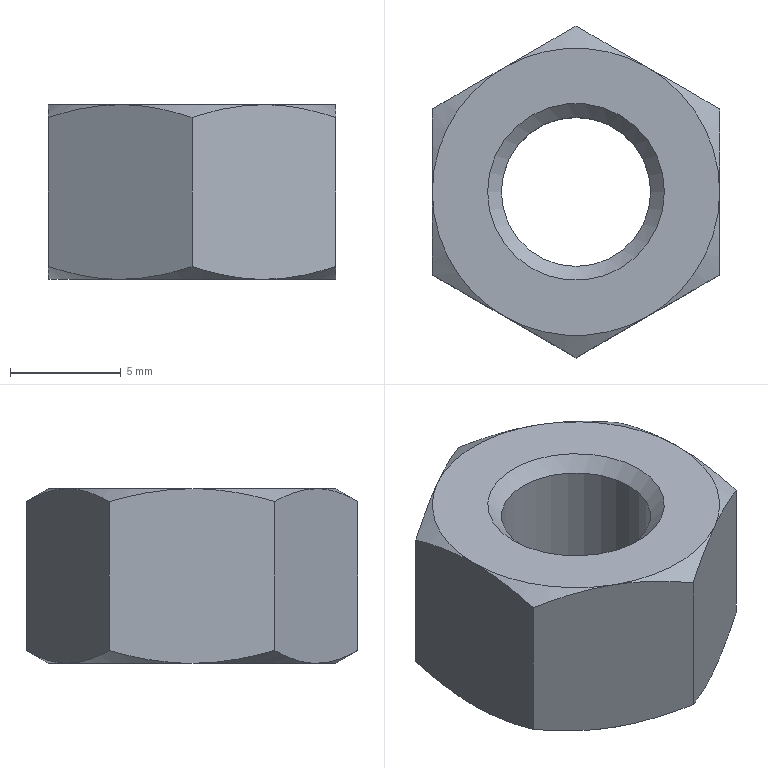Part | NX | features BREP 1, DATUM_CSYS 1 | 1 solid | 23 faces | box 13 x 15.011 x 7.9 mm | volume 859.913 mm3 | cone 14 | plane 8 | cylinder 1 | commonest cylinder face diameters 6.75 x1
STEP:
#1=CARTESIAN_POINT('',(-3.25,5.629,0.));
#2=VERTEX_POINT('',#1);
#3=CARTESIAN_POINT('',(-6.5,0.,0.));
#4=VERTEX_POINT('',#3);
#5=CARTESIAN_POINT('',(0.,0.,0.));
#6=DIRECTION('',(0.,0.,1.));
#7=DIRECTION('',(-0.5,0.866,0.));
#8=AXIS2_PLACEMENT_3D('',#5,#6,#7);
#9=CIRCLE('',#8,6.5);
#10=EDGE_CURVE('',#2,#4,#9,.T.);
#11=ORIENTED_EDGE('',*,*,#10,.F.);
#12=CARTESIAN_POINT('',(3.25,5.629,0.));
#13=VERTEX_POINT('',#12);
#14=CARTESIAN_POINT('',(0.,0.,0.));
#15=DIRECTION('',(0.,0.,1.));
#16=DIRECTION('',(0.5,0.866,0.));
#17=AXIS2_PLACEMENT_3D('',#14,#15,#16);
#18=CIRCLE('',#17,6.5);
#19=EDGE_CURVE('',#13,#2,#18,.T.);
#20=ORIENTED_EDGE('',*,*,#19,.F.);
#21=CARTESIAN_POINT('',(6.5,0.000000015,0.));
#22=VERTEX_POINT('',#21);
#23=CARTESIAN_POINT('',(0.,0.,0.));
#24=DIRECTION('',(0.,0.,1.));
#25=DIRECTION('',(1.,0.,0.));
#26=AXIS2_PLACEMENT_3D('',#23,#24,#25);
#27=CIRCLE('',#26,6.5);
#28=EDGE_CURVE('',#22,#13,#27,.T.);
#29=ORIENTED_EDGE('',*,*,#28,.F.);
#30=CARTESIAN_POINT('',(3.25,-5.629,0.));
#31=VERTEX_POINT('',#30);
#32=CARTESIAN_POINT('',(0.,0.,0.));
#33=DIRECTION('',(0.,0.,1.));
#34=DIRECTION('',(0.5,-0.866,0.));
#35=AXIS2_PLACEMENT_3D('',#32,#33,#34);
#36=CIRCLE('',#35,6.5);
#37=EDGE_CURVE('',#31,#22,#36,.T.);
#38=ORIENTED_EDGE('',*,*,#37,.F.);
#39=CARTESIAN_POINT('',(-3.25,-5.629,0.));
#40=VERTEX_POINT('',#39);
#41=CARTESIAN_POINT('',(0.,0.,0.));
#42=DIRECTION('',(0.,0.,1.));
#43=DIRECTION('',(-0.5,-0.866,0.));
#44=AXIS2_PLACEMENT_3D('',#41,#42,#43);
#45=CIRCLE('',#44,6.5);
#46=EDGE_CURVE('',#40,#31,#45,.T.);
#47=ORIENTED_EDGE('',*,*,#46,.F.);
#48=CARTESIAN_POINT('',(0.,0.,0.));
#49=DIRECTION('',(0.,0.,1.));
#50=DIRECTION('',(-1.,0.,0.));
#51=AXIS2_PLACEMENT_3D('',#48,#49,#50);
#52=CIRCLE('',#51,6.5);
#53=EDGE_CURVE('',#4,#40,#52,.T.);
#54=ORIENTED_EDGE('',*,*,#53,.F.);
#55=EDGE_LOOP('',(#11,#20,#29,#38,#47,#54));
#56=FACE_BOUND('',#55,.T.);
#57=CARTESIAN_POINT('',(4.,0.,0.));
#58=VERTEX_POINT('',#57);
#59=CARTESIAN_POINT('',(0.,0.,0.));
#60=DIRECTION('',(0.,0.,1.));
#61=DIRECTION('',(1.,0.,0.));
#62=AXIS2_PLACEMENT_3D('',#59,#60,#61);
#63=CIRCLE('',#62,4.);
#64=EDGE_CURVE('',#58,#58,#63,.T.);
#65=ORIENTED_EDGE('',*,*,#64,.T.);
#66=EDGE_LOOP('',(#65));
#67=FACE_BOUND('',#66,.T.);
#68=CARTESIAN_POINT('',(1.006,0.,0.));
#69=DIRECTION('',(0.,0.,1.));
#70=DIRECTION('',(-1.,0.,0.));
#71=AXIS2_PLACEMENT_3D('',#68,#69,#70);
#72=PLANE('',#71);
#73=ADVANCED_FACE('',(#56,#67),#72,.F.);
#74=CARTESIAN_POINT('',(6.5,0.,7.9));
#75=VERTEX_POINT('',#74);
#76=CARTESIAN_POINT('',(3.25,-5.629,7.9));
#77=VERTEX_POINT('',#76);
#78=CARTESIAN_POINT('',(0.,0.,7.9));
#79=DIRECTION('',(0.,0.,-1.));
#80=DIRECTION('',(1.,0.,0.));
#81=AXIS2_PLACEMENT_3D('',#78,#79,#80);
#82=CIRCLE('',#81,6.5);
#83=EDGE_CURVE('',#75,#77,#82,.T.);
#84=ORIENTED_EDGE('',*,*,#83,.F.);
#85=CARTESIAN_POINT('',(3.25,5.629,7.9));
#86=VERTEX_POINT('',#85);
#87=CARTESIAN_POINT('',(0.,0.,7.9));
#88=DIRECTION('',(0.,0.,-1.));
#89=DIRECTION('',(0.5,0.866,0.));
#90=AXIS2_PLACEMENT_3D('',#87,#88,#89);
#91=CIRCLE('',#90,6.5);
#92=EDGE_CURVE('',#86,#75,#91,.T.);
#93=ORIENTED_EDGE('',*,*,#92,.F.);
#94=CARTESIAN_POINT('',(-3.25,5.629,7.9));
#95=VERTEX_POINT('',#94);
#96=CARTESIAN_POINT('',(0.,0.,7.9));
#97=DIRECTION('',(0.,0.,-1.));
#98=DIRECTION('',(-0.5,0.866,0.));
#99=AXIS2_PLACEMENT_3D('',#96,#97,#98);
#100=CIRCLE('',#99,6.5);
#101=EDGE_CURVE('',#95,#86,#100,.T.);
#102=ORIENTED_EDGE('',*,*,#101,.F.);
#103=CARTESIAN_POINT('',(-6.5,0.000000016,7.9));
#104=VERTEX_POINT('',#103);
#105=CARTESIAN_POINT('',(0.,0.,7.9));
#106=DIRECTION('',(0.,0.,-1.));
#107=DIRECTION('',(-1.,0.,0.));
#108=AXIS2_PLACEMENT_3D('',#105,#106,#107);
#109=CIRCLE('',#108,6.5);
#110=EDGE_CURVE('',#104,#95,#109,.T.);
#111=ORIENTED_EDGE('',*,*,#110,.F.);
#112=CARTESIAN_POINT('',(-3.25,-5.629,7.9));
#113=VERTEX_POINT('',#112);
#114=CARTESIAN_POINT('',(0.,0.,7.9));
#115=DIRECTION('',(0.,0.,-1.));
#116=DIRECTION('',(-0.5,-0.866,0.));
#117=AXIS2_PLACEMENT_3D('',#114,#115,#116);
#118=CIRCLE('',#117,6.5);
#119=EDGE_CURVE('',#113,#104,#118,.T.);
#120=ORIENTED_EDGE('',*,*,#119,.F.);
#121=CARTESIAN_POINT('',(0.,0.,7.9));
#122=DIRECTION('',(0.,0.,-1.));
#123=DIRECTION('',(0.5,-0.866,0.));
#124=AXIS2_PLACEMENT_3D('',#121,#122,#123);
#125=CIRCLE('',#124,6.5);
#126=EDGE_CURVE('',#77,#113,#125,.T.);
#127=ORIENTED_EDGE('',*,*,#126,.F.);
#128=EDGE_LOOP('',(#84,#93,#102,#111,#120,#127));
#129=FACE_BOUND('',#128,.T.);
#130=CARTESIAN_POINT('',(4.,0.,7.9));
#131=VERTEX_POINT('',#130);
#132=CARTESIAN_POINT('',(0.,0.,7.9));
#133=DIRECTION('',(0.,0.,1.));
#134=DIRECTION('',(1.,0.,0.));
#135=AXIS2_PLACEMENT_3D('',#132,#133,#134);
#136=CIRCLE('',#135,4.);
#137=EDGE_CURVE('',#131,#131,#136,.T.);
#138=ORIENTED_EDGE('',*,*,#137,.F.);
#139=EDGE_LOOP('',(#138));
#140=FACE_BOUND('',#139,.T.);
#141=CARTESIAN_POINT('',(1.006,0.,7.9));
#142=DIRECTION('',(0.,0.,1.));
#143=DIRECTION('',(-1.,0.,0.));
#144=AXIS2_PLACEMENT_3D('',#141,#142,#143);
#145=PLANE('',#144);
#146=ADVANCED_FACE('',(#129,#140),#145,.T.);
#147=CARTESIAN_POINT('',(0.,7.506,7.319));
#148=VERTEX_POINT('',#147);
#149=CARTESIAN_POINT('',(3.25,5.629,7.9));
#150=CARTESIAN_POINT('',(2.141,6.27,7.9));
#151=CARTESIAN_POINT('',(1.062,6.892,7.673));
#152=CARTESIAN_POINT('',(0.,7.506,7.319));
#153=B_SPLINE_CURVE_WITH_KNOTS('',3,(#149,#150,#151,#152),.UNSPECIFIED.,.F.,.F.,(4,4),(0.,0.003797),.UNSPECIFIED.);
#154=EDGE_CURVE('',#86,#148,#153,.T.);
#155=ORIENTED_EDGE('',*,*,#154,.F.);
#156=CARTESIAN_POINT('',(6.5,3.753,7.319));
#157=VERTEX_POINT('',#156);
#158=CARTESIAN_POINT('',(6.5,3.753,7.319));
#159=CARTESIAN_POINT('',(5.438,4.366,7.673));
#160=CARTESIAN_POINT('',(4.359,4.989,7.9));
#161=CARTESIAN_POINT('',(3.25,5.629,7.9));
#162=B_SPLINE_CURVE_WITH_KNOTS('',3,(#158,#159,#160,#161),.UNSPECIFIED.,.F.,.F.,(4,4),(0.,0.003797),.UNSPECIFIED.);
#163=EDGE_CURVE('',#157,#86,#162,.T.);
#164=ORIENTED_EDGE('',*,*,#163,.F.);
#165=CARTESIAN_POINT('',(6.5,3.753,0.5806));
#166=VERTEX_POINT('',#165);
#167=CARTESIAN_POINT('',(6.5,3.753,0.5806));
#168=DIRECTION('',(0.,0.,1.));
#169=VECTOR('',#168,1000.);
#170=LINE('',#167,#169);
#171=EDGE_CURVE('',#166,#157,#170,.T.);
#172=ORIENTED_EDGE('',*,*,#171,.F.);
#173=CARTESIAN_POINT('',(3.25,5.629,0.));
#174=CARTESIAN_POINT('',(4.359,4.989,0.));
#175=CARTESIAN_POINT('',(5.438,4.366,0.2266));
#176=CARTESIAN_POINT('',(6.5,3.753,0.5806));
#177=B_SPLINE_CURVE_WITH_KNOTS('',3,(#173,#174,#175,#176),.UNSPECIFIED.,.F.,.F.,(4,4),(0.,0.003797),.UNSPECIFIED.);
#178=EDGE_CURVE('',#13,#166,#177,.T.);
#179=ORIENTED_EDGE('',*,*,#178,.F.);
#180=CARTESIAN_POINT('',(0.,7.506,0.5806));
#181=VERTEX_POINT('',#180);
#182=CARTESIAN_POINT('',(0.,7.506,0.5806));
#183=CARTESIAN_POINT('',(1.062,6.892,0.2266));
#184=CARTESIAN_POINT('',(2.141,6.27,0.));
#185=CARTESIAN_POINT('',(3.25,5.629,0.));
#186=B_SPLINE_CURVE_WITH_KNOTS('',3,(#182,#183,#184,#185),.UNSPECIFIED.,.F.,.F.,(4,4),(0.,0.003797),.UNSPECIFIED.);
#187=EDGE_CURVE('',#181,#13,#186,.T.);
#188=ORIENTED_EDGE('',*,*,#187,.F.);
#189=CARTESIAN_POINT('',(0.,7.506,0.5806));
#190=DIRECTION('',(0.,0.,1.));
#191=VECTOR('',#190,1000.);
#192=LINE('',#189,#191);
#193=EDGE_CURVE('',#181,#148,#192,.T.);
#194=ORIENTED_EDGE('',*,*,#193,.T.);
#195=EDGE_LOOP('',(#155,#164,#172,#179,#188,#194));
#196=FACE_BOUND('',#195,.T.);
#197=CARTESIAN_POINT('',(3.25,5.629,3.95));
#198=DIRECTION('',(0.5,0.866,0.));
#199=DIRECTION('',(0.866,-0.5,0.));
#200=AXIS2_PLACEMENT_3D('',#197,#198,#199);
#201=PLANE('',#200);
#202=ADVANCED_FACE('',(#196),#201,.T.);
#203=CARTESIAN_POINT('',(-6.5,3.753,7.319));
#204=VERTEX_POINT('',#203);
#205=CARTESIAN_POINT('',(-3.25,5.629,7.9));
#206=CARTESIAN_POINT('',(-4.359,4.989,7.9));
#207=CARTESIAN_POINT('',(-5.438,4.366,7.673));
#208=CARTESIAN_POINT('',(-6.5,3.753,7.319));
#209=B_SPLINE_CURVE_WITH_KNOTS('',3,(#205,#206,#207,#208),.UNSPECIFIED.,.F.,.F.,(4,4),(0.,0.003797),.UNSPECIFIED.);
#210=EDGE_CURVE('',#95,#204,#209,.T.);
#211=ORIENTED_EDGE('',*,*,#210,.F.);
#212=CARTESIAN_POINT('',(0.,7.506,7.319));
#213=CARTESIAN_POINT('',(-1.062,6.892,7.673));
#214=CARTESIAN_POINT('',(-2.141,6.27,7.9));
#215=CARTESIAN_POINT('',(-3.25,5.629,7.9));
#216=B_SPLINE_CURVE_WITH_KNOTS('',3,(#212,#213,#214,#215),.UNSPECIFIED.,.F.,.F.,(4,4),(0.,0.003797),.UNSPECIFIED.);
#217=EDGE_CURVE('',#148,#95,#216,.T.);
#218=ORIENTED_EDGE('',*,*,#217,.F.);
#219=ORIENTED_EDGE('',*,*,#193,.F.);
#220=CARTESIAN_POINT('',(-3.25,5.629,0.));
#221=CARTESIAN_POINT('',(-2.141,6.27,-0.000000003));
#222=CARTESIAN_POINT('',(-1.062,6.892,0.2266));
#223=CARTESIAN_POINT('',(0.,7.506,0.5806));
#224=B_SPLINE_CURVE_WITH_KNOTS('',3,(#220,#221,#222,#223),.UNSPECIFIED.,.F.,.F.,(4,4),(0.,0.003797),.UNSPECIFIED.);
#225=EDGE_CURVE('',#2,#181,#224,.T.);
#226=ORIENTED_EDGE('',*,*,#225,.F.);
#227=CARTESIAN_POINT('',(-6.5,3.753,0.5806));
#228=VERTEX_POINT('',#227);
#229=CARTESIAN_POINT('',(-6.5,3.753,0.5806));
#230=CARTESIAN_POINT('',(-5.438,4.366,0.2266));
#231=CARTESIAN_POINT('',(-4.359,4.989,0.000000003));
#232=CARTESIAN_POINT('',(-3.25,5.629,0.));
#233=B_SPLINE_CURVE_WITH_KNOTS('',3,(#229,#230,#231,#232),.UNSPECIFIED.,.F.,.F.,(4,4),(0.,0.003797),.UNSPECIFIED.);
#234=EDGE_CURVE('',#228,#2,#233,.T.);
#235=ORIENTED_EDGE('',*,*,#234,.F.);
#236=CARTESIAN_POINT('',(-6.5,3.753,0.5806));
#237=DIRECTION('',(0.,0.,1.));
#238=VECTOR('',#237,1000.);
#239=LINE('',#236,#238);
#240=EDGE_CURVE('',#228,#204,#239,.T.);
#241=ORIENTED_EDGE('',*,*,#240,.T.);
#242=EDGE_LOOP('',(#211,#218,#219,#226,#235,#241));
#243=FACE_BOUND('',#242,.T.);
#244=CARTESIAN_POINT('',(-3.25,5.629,3.95));
#245=DIRECTION('',(-0.5,0.866,0.));
#246=DIRECTION('',(0.866,0.5,0.));
#247=AXIS2_PLACEMENT_3D('',#244,#245,#246);
#248=PLANE('',#247);
#249=ADVANCED_FACE('',(#243),#248,.T.);
#250=CARTESIAN_POINT('',(-6.5,-3.753,7.319));
#251=VERTEX_POINT('',#250);
#252=CARTESIAN_POINT('',(-6.5,0.000000032,7.9));
#253=CARTESIAN_POINT('',(-6.5,-1.281,7.9));
#254=CARTESIAN_POINT('',(-6.5,-2.527,7.673));
#255=CARTESIAN_POINT('',(-6.5,-3.753,7.319));
#256=B_SPLINE_CURVE_WITH_KNOTS('',3,(#252,#253,#254,#255),.UNSPECIFIED.,.F.,.F.,(4,4),(0.,0.003797),.UNSPECIFIED.);
#257=EDGE_CURVE('',#104,#251,#256,.T.);
#258=ORIENTED_EDGE('',*,*,#257,.F.);
#259=CARTESIAN_POINT('',(-6.5,3.753,7.319));
#260=CARTESIAN_POINT('',(-6.5,2.527,7.673));
#261=CARTESIAN_POINT('',(-6.5,1.281,7.9));
#262=CARTESIAN_POINT('',(-6.5,0.000000032,7.9));
#263=B_SPLINE_CURVE_WITH_KNOTS('',3,(#259,#260,#261,#262),.UNSPECIFIED.,.F.,.F.,(4,4),(0.,0.003797),.UNSPECIFIED.);
#264=EDGE_CURVE('',#204,#104,#263,.T.);
#265=ORIENTED_EDGE('',*,*,#264,.F.);
#266=ORIENTED_EDGE('',*,*,#240,.F.);
#267=CARTESIAN_POINT('',(-6.5,0.,0.));
#268=CARTESIAN_POINT('',(-6.5,1.281,0.));
#269=CARTESIAN_POINT('',(-6.5,2.527,0.2266));
#270=CARTESIAN_POINT('',(-6.5,3.753,0.5806));
#271=B_SPLINE_CURVE_WITH_KNOTS('',3,(#267,#268,#269,#270),.UNSPECIFIED.,.F.,.F.,(4,4),(0.,0.003797),.UNSPECIFIED.);
#272=EDGE_CURVE('',#4,#228,#271,.T.);
#273=ORIENTED_EDGE('',*,*,#272,.F.);
#274=CARTESIAN_POINT('',(-6.5,-3.753,0.5806));
#275=VERTEX_POINT('',#274);
#276=CARTESIAN_POINT('',(-6.5,-3.753,0.5806));
#277=CARTESIAN_POINT('',(-6.5,-2.527,0.2266));
#278=CARTESIAN_POINT('',(-6.5,-1.281,0.));
#279=CARTESIAN_POINT('',(-6.5,0.,0.));
#280=B_SPLINE_CURVE_WITH_KNOTS('',3,(#276,#277,#278,#279),.UNSPECIFIED.,.F.,.F.,(4,4),(0.,0.003797),.UNSPECIFIED.);
#281=EDGE_CURVE('',#275,#4,#280,.T.);
#282=ORIENTED_EDGE('',*,*,#281,.F.);
#283=CARTESIAN_POINT('',(-6.5,-3.753,0.5806));
#284=DIRECTION('',(0.,0.,1.));
#285=VECTOR('',#284,1000.);
#286=LINE('',#283,#285);
#287=EDGE_CURVE('',#275,#251,#286,.T.);
#288=ORIENTED_EDGE('',*,*,#287,.T.);
#289=EDGE_LOOP('',(#258,#265,#266,#273,#282,#288));
#290=FACE_BOUND('',#289,.T.);
#291=CARTESIAN_POINT('',(-6.5,0.,3.95));
#292=DIRECTION('',(-1.,0.,0.));
#293=DIRECTION('',(0.,1.,0.));
#294=AXIS2_PLACEMENT_3D('',#291,#292,#293);
#295=PLANE('',#294);
#296=ADVANCED_FACE('',(#290),#295,.T.);
#297=CARTESIAN_POINT('',(0.,-7.506,7.319));
#298=VERTEX_POINT('',#297);
#299=CARTESIAN_POINT('',(-3.25,-5.629,7.9));
#300=CARTESIAN_POINT('',(-2.141,-6.27,7.9));
#301=CARTESIAN_POINT('',(-1.062,-6.892,7.673));
#302=CARTESIAN_POINT('',(0.,-7.506,7.319));
#303=B_SPLINE_CURVE_WITH_KNOTS('',3,(#299,#300,#301,#302),.UNSPECIFIED.,.F.,.F.,(4,4),(0.,0.003797),.UNSPECIFIED.);
#304=EDGE_CURVE('',#113,#298,#303,.T.);
#305=ORIENTED_EDGE('',*,*,#304,.F.);
#306=CARTESIAN_POINT('',(-6.5,-3.753,7.319));
#307=CARTESIAN_POINT('',(-5.438,-4.366,7.673));
#308=CARTESIAN_POINT('',(-4.359,-4.989,7.9));
#309=CARTESIAN_POINT('',(-3.25,-5.629,7.9));
#310=B_SPLINE_CURVE_WITH_KNOTS('',3,(#306,#307,#308,#309),.UNSPECIFIED.,.F.,.F.,(4,4),(0.,0.003797),.UNSPECIFIED.);
#311=EDGE_CURVE('',#251,#113,#310,.T.);
#312=ORIENTED_EDGE('',*,*,#311,.F.);
#313=ORIENTED_EDGE('',*,*,#287,.F.);
#314=CARTESIAN_POINT('',(-3.25,-5.629,0.));
#315=CARTESIAN_POINT('',(-4.359,-4.989,-0.000000001));
#316=CARTESIAN_POINT('',(-5.438,-4.366,0.2266));
#317=CARTESIAN_POINT('',(-6.5,-3.753,0.5806));
#318=B_SPLINE_CURVE_WITH_KNOTS('',3,(#314,#315,#316,#317),.UNSPECIFIED.,.F.,.F.,(4,4),(0.,0.003797),.UNSPECIFIED.);
#319=EDGE_CURVE('',#40,#275,#318,.T.);
#320=ORIENTED_EDGE('',*,*,#319,.F.);
#321=CARTESIAN_POINT('',(0.,-7.506,0.5806));
#322=VERTEX_POINT('',#321);
#323=CARTESIAN_POINT('',(0.,-7.506,0.5806));
#324=CARTESIAN_POINT('',(-1.062,-6.892,0.2266));
#325=CARTESIAN_POINT('',(-2.141,-6.27,0.000000001));
#326=CARTESIAN_POINT('',(-3.25,-5.629,0.));
#327=B_SPLINE_CURVE_WITH_KNOTS('',3,(#323,#324,#325,#326),.UNSPECIFIED.,.F.,.F.,(4,4),(0.,0.003797),.UNSPECIFIED.);
#328=EDGE_CURVE('',#322,#40,#327,.T.);
#329=ORIENTED_EDGE('',*,*,#328,.F.);
#330=CARTESIAN_POINT('',(0.,-7.506,0.5806));
#331=DIRECTION('',(0.,0.,1.));
#332=VECTOR('',#331,1000.);
#333=LINE('',#330,#332);
#334=EDGE_CURVE('',#322,#298,#333,.T.);
#335=ORIENTED_EDGE('',*,*,#334,.T.);
#336=EDGE_LOOP('',(#305,#312,#313,#320,#329,#335));
#337=FACE_BOUND('',#336,.T.);
#338=CARTESIAN_POINT('',(-3.25,-5.629,3.95));
#339=DIRECTION('',(-0.5,-0.866,0.));
#340=DIRECTION('',(-0.866,0.5,0.));
#341=AXIS2_PLACEMENT_3D('',#338,#339,#340);
#342=PLANE('',#341);
#343=ADVANCED_FACE('',(#337),#342,.T.);
#344=CARTESIAN_POINT('',(6.5,-3.753,7.319));
#345=VERTEX_POINT('',#344);
#346=CARTESIAN_POINT('',(3.25,-5.629,7.9));
#347=CARTESIAN_POINT('',(4.359,-4.989,7.9));
#348=CARTESIAN_POINT('',(5.438,-4.366,7.673));
#349=CARTESIAN_POINT('',(6.5,-3.753,7.319));
#350=B_SPLINE_CURVE_WITH_KNOTS('',3,(#346,#347,#348,#349),.UNSPECIFIED.,.F.,.F.,(4,4),(0.,0.003797),.UNSPECIFIED.);
#351=EDGE_CURVE('',#77,#345,#350,.T.);
#352=ORIENTED_EDGE('',*,*,#351,.F.);
#353=CARTESIAN_POINT('',(0.,-7.506,7.319));
#354=CARTESIAN_POINT('',(1.062,-6.892,7.673));
#355=CARTESIAN_POINT('',(2.141,-6.27,7.9));
#356=CARTESIAN_POINT('',(3.25,-5.629,7.9));
#357=B_SPLINE_CURVE_WITH_KNOTS('',3,(#353,#354,#355,#356),.UNSPECIFIED.,.F.,.F.,(4,4),(0.,0.003797),.UNSPECIFIED.);
#358=EDGE_CURVE('',#298,#77,#357,.T.);
#359=ORIENTED_EDGE('',*,*,#358,.F.);
#360=ORIENTED_EDGE('',*,*,#334,.F.);
#361=CARTESIAN_POINT('',(3.25,-5.629,0.));
#362=CARTESIAN_POINT('',(2.141,-6.27,-0.000000004));
#363=CARTESIAN_POINT('',(1.062,-6.892,0.2266));
#364=CARTESIAN_POINT('',(0.,-7.506,0.5806));
#365=B_SPLINE_CURVE_WITH_KNOTS('',3,(#361,#362,#363,#364),.UNSPECIFIED.,.F.,.F.,(4,4),(0.,0.003797),.UNSPECIFIED.);
#366=EDGE_CURVE('',#31,#322,#365,.T.);
#367=ORIENTED_EDGE('',*,*,#366,.F.);
#368=CARTESIAN_POINT('',(6.5,-3.753,0.5806));
#369=VERTEX_POINT('',#368);
#370=CARTESIAN_POINT('',(6.5,-3.753,0.5806));
#371=CARTESIAN_POINT('',(5.438,-4.366,0.2266));
#372=CARTESIAN_POINT('',(4.359,-4.989,0.000000004));
#373=CARTESIAN_POINT('',(3.25,-5.629,0.));
#374=B_SPLINE_CURVE_WITH_KNOTS('',3,(#370,#371,#372,#373),.UNSPECIFIED.,.F.,.F.,(4,4),(0.,0.003797),.UNSPECIFIED.);
#375=EDGE_CURVE('',#369,#31,#374,.T.);
#376=ORIENTED_EDGE('',*,*,#375,.F.);
#377=CARTESIAN_POINT('',(6.5,-3.753,0.5806));
#378=DIRECTION('',(0.,0.,1.));
#379=VECTOR('',#378,1000.);
#380=LINE('',#377,#379);
#381=EDGE_CURVE('',#369,#345,#380,.T.);
#382=ORIENTED_EDGE('',*,*,#381,.T.);
#383=EDGE_LOOP('',(#352,#359,#360,#367,#376,#382));
#384=FACE_BOUND('',#383,.T.);
#385=CARTESIAN_POINT('',(3.25,-5.629,3.95));
#386=DIRECTION('',(0.5,-0.866,0.));
#387=DIRECTION('',(-0.866,-0.5,0.));
#388=AXIS2_PLACEMENT_3D('',#385,#386,#387);
#389=PLANE('',#388);
#390=ADVANCED_FACE('',(#384),#389,.T.);
#391=CARTESIAN_POINT('',(6.5,0.,7.9));
#392=CARTESIAN_POINT('',(6.5,1.281,7.9));
#393=CARTESIAN_POINT('',(6.5,2.527,7.673));
#394=CARTESIAN_POINT('',(6.5,3.753,7.319));
#395=B_SPLINE_CURVE_WITH_KNOTS('',3,(#391,#392,#393,#394),.UNSPECIFIED.,.F.,.F.,(4,4),(0.,0.003797),.UNSPECIFIED.);
#396=EDGE_CURVE('',#75,#157,#395,.T.);
#397=ORIENTED_EDGE('',*,*,#396,.F.);
#398=CARTESIAN_POINT('',(6.5,-3.753,7.319));
#399=CARTESIAN_POINT('',(6.5,-2.527,7.673));
#400=CARTESIAN_POINT('',(6.5,-1.281,7.9));
#401=CARTESIAN_POINT('',(6.5,0.,7.9));
#402=B_SPLINE_CURVE_WITH_KNOTS('',3,(#398,#399,#400,#401),.UNSPECIFIED.,.F.,.F.,(4,4),(0.,0.003797),.UNSPECIFIED.);
#403=EDGE_CURVE('',#345,#75,#402,.T.);
#404=ORIENTED_EDGE('',*,*,#403,.F.);
#405=ORIENTED_EDGE('',*,*,#381,.F.);
#406=CARTESIAN_POINT('',(6.5,0.00000003,0.));
#407=CARTESIAN_POINT('',(6.5,-1.281,-0.000000003));
#408=CARTESIAN_POINT('',(6.5,-2.527,0.2266));
#409=CARTESIAN_POINT('',(6.5,-3.753,0.5806));
#410=B_SPLINE_CURVE_WITH_KNOTS('',3,(#406,#407,#408,#409),.UNSPECIFIED.,.F.,.F.,(4,4),(0.,0.003797),.UNSPECIFIED.);
#411=EDGE_CURVE('',#22,#369,#410,.T.);
#412=ORIENTED_EDGE('',*,*,#411,.F.);
#413=CARTESIAN_POINT('',(6.5,3.753,0.5806));
#414=CARTESIAN_POINT('',(6.5,2.527,0.2266));
#415=CARTESIAN_POINT('',(6.5,1.281,0.000000003));
#416=CARTESIAN_POINT('',(6.5,0.00000003,0.));
#417=B_SPLINE_CURVE_WITH_KNOTS('',3,(#413,#414,#415,#416),.UNSPECIFIED.,.F.,.F.,(4,4),(0.,0.003797),.UNSPECIFIED.);
#418=EDGE_CURVE('',#166,#22,#417,.T.);
#419=ORIENTED_EDGE('',*,*,#418,.F.);
#420=ORIENTED_EDGE('',*,*,#171,.T.);
#421=EDGE_LOOP('',(#397,#404,#405,#412,#419,#420));
#422=FACE_BOUND('',#421,.T.);
#423=CARTESIAN_POINT('',(6.5,0.,3.95));
#424=DIRECTION('',(1.,0.,0.));
#425=DIRECTION('',(0.,-1.,0.));
#426=AXIS2_PLACEMENT_3D('',#423,#424,#425);
#427=PLANE('',#426);
#428=ADVANCED_FACE('',(#422),#427,.T.);
#429=CARTESIAN_POINT('',(3.375,0.,0.625));
#430=VERTEX_POINT('',#429);
#431=CARTESIAN_POINT('',(3.375,0.,7.275));
#432=VERTEX_POINT('',#431);
#433=CARTESIAN_POINT('',(3.375,0.,0.625));
#434=DIRECTION('',(0.,0.,1.));
#435=VECTOR('',#434,1000.);
#436=LINE('',#433,#435);
#437=EDGE_CURVE('',#430,#432,#436,.T.);
#438=ORIENTED_EDGE('',*,*,#437,.F.);
#439=CARTESIAN_POINT('',(0.,0.,0.625));
#440=DIRECTION('',(0.,0.,1.));
#441=DIRECTION('',(1.,0.,0.));
#442=AXIS2_PLACEMENT_3D('',#439,#440,#441);
#443=CIRCLE('',#442,3.375);
#444=EDGE_CURVE('',#430,#430,#443,.T.);
#445=ORIENTED_EDGE('',*,*,#444,.F.);
#446=ORIENTED_EDGE('',*,*,#437,.T.);
#447=CARTESIAN_POINT('',(0.,0.,7.275));
#448=DIRECTION('',(0.,0.,1.));
#449=DIRECTION('',(1.,0.,0.));
#450=AXIS2_PLACEMENT_3D('',#447,#448,#449);
#451=CIRCLE('',#450,3.375);
#452=EDGE_CURVE('',#432,#432,#451,.T.);
#453=ORIENTED_EDGE('',*,*,#452,.T.);
#454=EDGE_LOOP('',(#438,#445,#446,#453));
#455=FACE_BOUND('',#454,.T.);
#456=CARTESIAN_POINT('',(0.,0.,0.));
#457=DIRECTION('',(0.,0.,1.));
#458=DIRECTION('',(-1.,0.,0.));
#459=AXIS2_PLACEMENT_3D('',#456,#457,#458);
#460=CYLINDRICAL_SURFACE('',#459,3.375);
#461=ADVANCED_FACE('',(#455),#460,.F.);
#462=ORIENTED_EDGE('',*,*,#64,.F.);
#463=CARTESIAN_POINT('',(3.375,0.,0.625));
#464=DIRECTION('',(0.7071,0.,-0.7071));
#465=VECTOR('',#464,1000.);
#466=LINE('',#463,#465);
#467=EDGE_CURVE('',#430,#58,#466,.T.);
#468=ORIENTED_EDGE('',*,*,#467,.F.);
#469=ORIENTED_EDGE('',*,*,#444,.T.);
#470=ORIENTED_EDGE('',*,*,#467,.T.);
#471=EDGE_LOOP('',(#462,#468,#469,#470));
#472=FACE_BOUND('',#471,.T.);
#473=CARTESIAN_POINT('',(0.,0.,0.625));
#474=DIRECTION('',(0.,0.,-1.));
#475=DIRECTION('',(-1.,0.,0.));
#476=AXIS2_PLACEMENT_3D('',#473,#474,#475);
#477=CONICAL_SURFACE('',#476,3.375,0.7854);
#478=ADVANCED_FACE('',(#472),#477,.F.);
#479=ORIENTED_EDGE('',*,*,#452,.F.);
#480=CARTESIAN_POINT('',(4.,0.,7.9));
#481=DIRECTION('',(-0.7071,0.,-0.7071));
#482=VECTOR('',#481,1000.);
#483=LINE('',#480,#482);
#484=EDGE_CURVE('',#131,#432,#483,.T.);
#485=ORIENTED_EDGE('',*,*,#484,.F.);
#486=ORIENTED_EDGE('',*,*,#137,.T.);
#487=ORIENTED_EDGE('',*,*,#484,.T.);
#488=EDGE_LOOP('',(#479,#485,#486,#487));
#489=FACE_BOUND('',#488,.T.);
#490=CARTESIAN_POINT('',(0.,0.,7.275));
#491=DIRECTION('',(0.,0.,1.));
#492=DIRECTION('',(-1.,0.,0.));
#493=AXIS2_PLACEMENT_3D('',#490,#491,#492);
#494=CONICAL_SURFACE('',#493,3.375,0.7854);
#495=ADVANCED_FACE('',(#489),#494,.F.);
#496=ORIENTED_EDGE('',*,*,#154,.T.);
#497=ORIENTED_EDGE('',*,*,#217,.T.);
#498=ORIENTED_EDGE('',*,*,#101,.T.);
#499=EDGE_LOOP('',(#496,#497,#498));
#500=FACE_BOUND('',#499,.T.);
#501=CARTESIAN_POINT('',(0.,0.,7.9));
#502=DIRECTION('',(0.,0.,-1.));
#503=DIRECTION('',(0.,1.,0.));
#504=AXIS2_PLACEMENT_3D('',#501,#502,#503);
#505=CONICAL_SURFACE('',#504,6.5,1.047);
#506=ADVANCED_FACE('',(#500),#505,.T.);
#507=ORIENTED_EDGE('',*,*,#396,.T.);
#508=ORIENTED_EDGE('',*,*,#163,.T.);
#509=ORIENTED_EDGE('',*,*,#92,.T.);
#510=EDGE_LOOP('',(#507,#508,#509));
#511=FACE_BOUND('',#510,.T.);
#512=CARTESIAN_POINT('',(0.,0.,7.9));
#513=DIRECTION('',(0.,0.,-1.));
#514=DIRECTION('',(0.,1.,0.));
#515=AXIS2_PLACEMENT_3D('',#512,#513,#514);
#516=CONICAL_SURFACE('',#515,6.5,1.047);
#517=ADVANCED_FACE('',(#511),#516,.T.);
#518=ORIENTED_EDGE('',*,*,#210,.T.);
#519=ORIENTED_EDGE('',*,*,#264,.T.);
#520=ORIENTED_EDGE('',*,*,#110,.T.);
#521=EDGE_LOOP('',(#518,#519,#520));
#522=FACE_BOUND('',#521,.T.);
#523=CARTESIAN_POINT('',(0.,0.,7.9));
#524=DIRECTION('',(0.,0.,-1.));
#525=DIRECTION('',(0.,1.,0.));
#526=AXIS2_PLACEMENT_3D('',#523,#524,#525);
#527=CONICAL_SURFACE('',#526,6.5,1.047);
#528=ADVANCED_FACE('',(#522),#527,.T.);
#529=ORIENTED_EDGE('',*,*,#257,.T.);
#530=ORIENTED_EDGE('',*,*,#311,.T.);
#531=ORIENTED_EDGE('',*,*,#119,.T.);
#532=EDGE_LOOP('',(#529,#530,#531));
#533=FACE_BOUND('',#532,.T.);
#534=CARTESIAN_POINT('',(0.,0.,7.9));
#535=DIRECTION('',(0.,0.,-1.));
#536=DIRECTION('',(0.,1.,0.));
#537=AXIS2_PLACEMENT_3D('',#534,#535,#536);
#538=CONICAL_SURFACE('',#537,6.5,1.047);
#539=ADVANCED_FACE('',(#533),#538,.T.);
#540=ORIENTED_EDGE('',*,*,#304,.T.);
#541=ORIENTED_EDGE('',*,*,#358,.T.);
#542=ORIENTED_EDGE('',*,*,#126,.T.);
#543=EDGE_LOOP('',(#540,#541,#542));
#544=FACE_BOUND('',#543,.T.);
#545=CARTESIAN_POINT('',(0.,0.,7.9));
#546=DIRECTION('',(0.,0.,-1.));
#547=DIRECTION('',(0.,1.,0.));
#548=AXIS2_PLACEMENT_3D('',#545,#546,#547);
#549=CONICAL_SURFACE('',#548,6.5,1.047);
#550=ADVANCED_FACE('',(#544),#549,.T.);
#551=ORIENTED_EDGE('',*,*,#351,.T.);
#552=ORIENTED_EDGE('',*,*,#403,.T.);
#553=ORIENTED_EDGE('',*,*,#83,.T.);
#554=EDGE_LOOP('',(#551,#552,#553));
#555=FACE_BOUND('',#554,.T.);
#556=CARTESIAN_POINT('',(0.,0.,7.9));
#557=DIRECTION('',(0.,0.,-1.));
#558=DIRECTION('',(0.,1.,0.));
#559=AXIS2_PLACEMENT_3D('',#556,#557,#558);
#560=CONICAL_SURFACE('',#559,6.5,1.047);
#561=ADVANCED_FACE('',(#555),#560,.T.);
#562=ORIENTED_EDGE('',*,*,#319,.T.);
#563=ORIENTED_EDGE('',*,*,#281,.T.);
#564=ORIENTED_EDGE('',*,*,#53,.T.);
#565=EDGE_LOOP('',(#562,#563,#564));
#566=FACE_BOUND('',#565,.T.);
#567=CARTESIAN_POINT('',(0.,0.,0.));
#568=DIRECTION('',(0.,0.,1.));
#569=DIRECTION('',(0.,-1.,0.));
#570=AXIS2_PLACEMENT_3D('',#567,#568,#569);
#571=CONICAL_SURFACE('',#570,6.5,1.047);
#572=ADVANCED_FACE('',(#566),#571,.T.);
#573=ORIENTED_EDGE('',*,*,#366,.T.);
#574=ORIENTED_EDGE('',*,*,#328,.T.);
#575=ORIENTED_EDGE('',*,*,#46,.T.);
#576=EDGE_LOOP('',(#573,#574,#575));
#577=FACE_BOUND('',#576,.T.);
#578=CARTESIAN_POINT('',(0.,0.,0.));
#579=DIRECTION('',(0.,0.,1.));
#580=DIRECTION('',(0.,-1.,0.));
#581=AXIS2_PLACEMENT_3D('',#578,#579,#580);
#582=CONICAL_SURFACE('',#581,6.5,1.047);
#583=ADVANCED_FACE('',(#577),#582,.T.);
#584=ORIENTED_EDGE('',*,*,#411,.T.);
#585=ORIENTED_EDGE('',*,*,#375,.T.);
#586=ORIENTED_EDGE('',*,*,#37,.T.);
#587=EDGE_LOOP('',(#584,#585,#586));
#588=FACE_BOUND('',#587,.T.);
#589=CARTESIAN_POINT('',(0.,0.,0.));
#590=DIRECTION('',(0.,0.,1.));
#591=DIRECTION('',(0.,-1.,0.));
#592=AXIS2_PLACEMENT_3D('',#589,#590,#591);
#593=CONICAL_SURFACE('',#592,6.5,1.047);
#594=ADVANCED_FACE('',(#588),#593,.T.);
#595=ORIENTED_EDGE('',*,*,#178,.T.);
#596=ORIENTED_EDGE('',*,*,#418,.T.);
#597=ORIENTED_EDGE('',*,*,#28,.T.);
#598=EDGE_LOOP('',(#595,#596,#597));
#599=FACE_BOUND('',#598,.T.);
#600=CARTESIAN_POINT('',(0.,0.,0.));
#601=DIRECTION('',(0.,0.,1.));
#602=DIRECTION('',(0.,-1.,0.));
#603=AXIS2_PLACEMENT_3D('',#600,#601,#602);
#604=CONICAL_SURFACE('',#603,6.5,1.047);
#605=ADVANCED_FACE('',(#599),#604,.T.);
#606=ORIENTED_EDGE('',*,*,#225,.T.);
#607=ORIENTED_EDGE('',*,*,#187,.T.);
#608=ORIENTED_EDGE('',*,*,#19,.T.);
#609=EDGE_LOOP('',(#606,#607,#608));
#610=FACE_BOUND('',#609,.T.);
#611=CARTESIAN_POINT('',(0.,0.,0.));
#612=DIRECTION('',(0.,0.,1.));
#613=DIRECTION('',(0.,-1.,0.));
#614=AXIS2_PLACEMENT_3D('',#611,#612,#613);
#615=CONICAL_SURFACE('',#614,6.5,1.047);
#616=ADVANCED_FACE('',(#610),#615,.T.);
#617=ORIENTED_EDGE('',*,*,#272,.T.);
#618=ORIENTED_EDGE('',*,*,#234,.T.);
#619=ORIENTED_EDGE('',*,*,#10,.T.);
#620=EDGE_LOOP('',(#617,#618,#619));
#621=FACE_BOUND('',#620,.T.);
#622=CARTESIAN_POINT('',(0.,0.,0.));
#623=DIRECTION('',(0.,0.,1.));
#624=DIRECTION('',(0.,-1.,0.));
#625=AXIS2_PLACEMENT_3D('',#622,#623,#624);
#626=CONICAL_SURFACE('',#625,6.5,1.047);
#627=ADVANCED_FACE('',(#621),#626,.T.);
#628=CLOSED_SHELL('',(#73,#146,#202,#249,#296,#343,#390,#428,#461,#478,#495,#506,#517,#528,#539,#550,#561,#572,#583,#594,#605,#616,#627));
#629=MANIFOLD_SOLID_BREP('',#628);
#630=(LENGTH_UNIT()NAMED_UNIT(*)SI_UNIT(.MILLI.,.METRE.));
#631=UNCERTAINTY_MEASURE_WITH_UNIT(LENGTH_MEASURE(0.0508),#630,'','');
#632=(NAMED_UNIT(*)PLANE_ANGLE_UNIT()SI_UNIT($,.RADIAN.));
#633=(NAMED_UNIT(*)SI_UNIT($,.STERADIAN.)SOLID_ANGLE_UNIT());
#634=(GEOMETRIC_REPRESENTATION_CONTEXT(3)GLOBAL_UNCERTAINTY_ASSIGNED_CONTEXT((#631))GLOBAL_UNIT_ASSIGNED_CONTEXT((#630,#632,#633))REPRESENTATION_CONTEXT('',''));
#635=ADVANCED_BREP_SHAPE_REPRESENTATION('',(#629),#634);